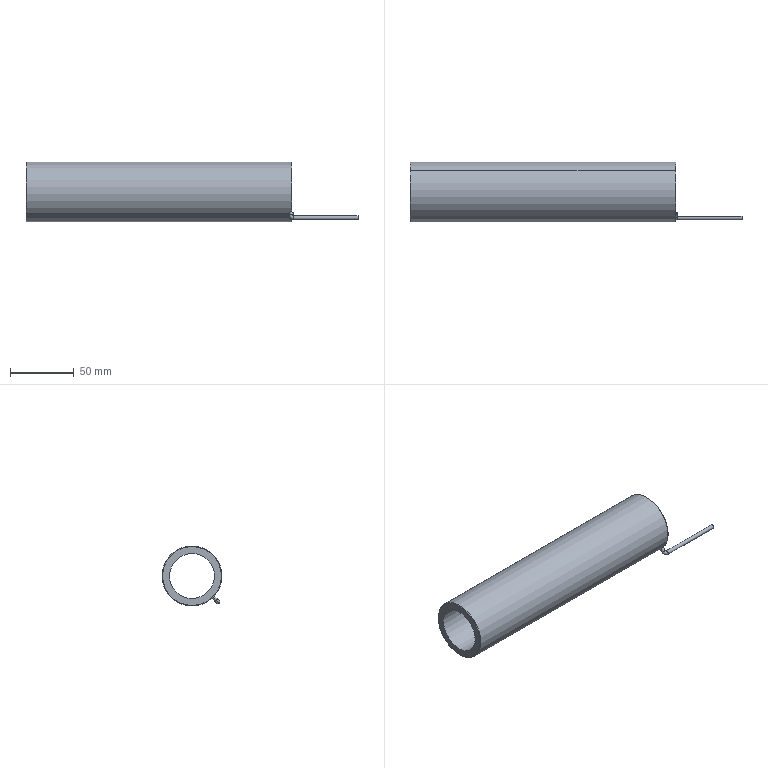Part | STEP file | Tube Heater_Bala35_toe-1 | 2 solids | 18 faces | box 259.756 x 47 x 47 mm | volume 158264 mm3 | cylinder 8 | torus 6 | plane 4 | commonest cylinder face diameters 3 x4 35.25 x2 47 x2